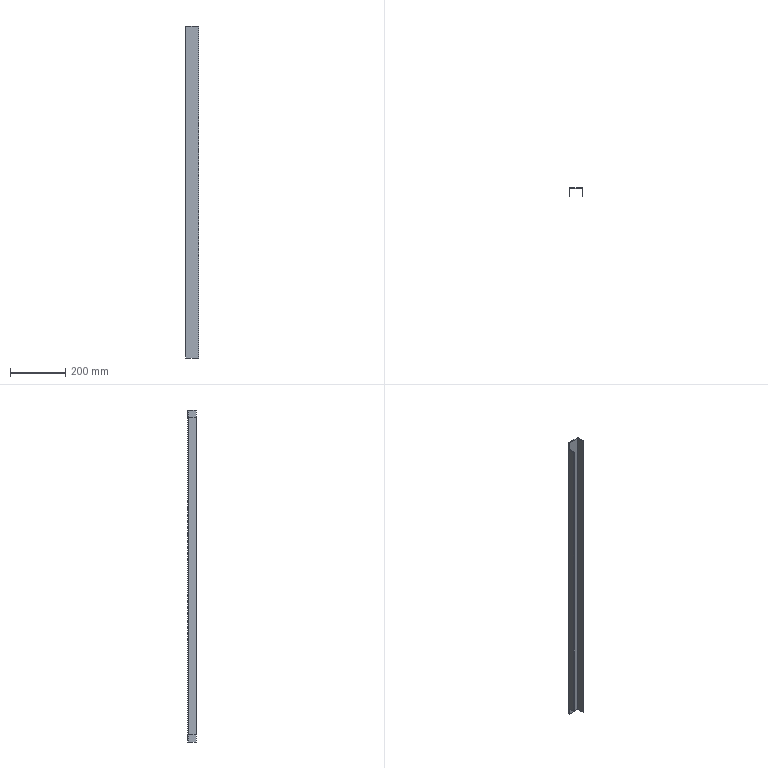Part | SolidWorks | 1 solid | 26 faces | box 50 x 30 x 1204 mm | volume 365931 mm3 | plane 22 | cylinder 4 | commonest cylinder face diameters 0.2 x2 6.2 x2
STEP:
#1=CARTESIAN_POINT('',(-25.,-3.1,575.));
#2=VERTEX_POINT('',#1);
#3=CARTESIAN_POINT('',(-25.,-30.,575.));
#4=VERTEX_POINT('',#3);
#5=CARTESIAN_POINT('',(-25.,-30.,575.));
#6=DIRECTION('',(0.,-1.,0.));
#7=VECTOR('',#6,1000.);
#8=LINE('',#5,#7);
#9=EDGE_CURVE('',#2,#4,#8,.T.);
#10=ORIENTED_EDGE('',*,*,#9,.F.);
#11=CARTESIAN_POINT('',(-25.,-3.1,-575.));
#12=VERTEX_POINT('',#11);
#13=CARTESIAN_POINT('',(-25.,-3.1,-602.));
#14=DIRECTION('',(0.,0.,1.));
#15=VECTOR('',#14,1000.);
#16=LINE('',#13,#15);
#17=EDGE_CURVE('',#12,#2,#16,.T.);
#18=ORIENTED_EDGE('',*,*,#17,.F.);
#19=CARTESIAN_POINT('',(-25.,-30.,-575.));
#20=VERTEX_POINT('',#19);
#21=CARTESIAN_POINT('',(-25.,-30.,-575.));
#22=DIRECTION('',(0.,-1.,0.));
#23=VECTOR('',#22,1000.);
#24=LINE('',#21,#23);
#25=EDGE_CURVE('',#12,#20,#24,.T.);
#26=ORIENTED_EDGE('',*,*,#25,.T.);
#27=CARTESIAN_POINT('',(-25.,-30.,-602.));
#28=DIRECTION('',(0.,0.,1.));
#29=VECTOR('',#28,1000.);
#30=LINE('',#27,#29);
#31=EDGE_CURVE('',#20,#4,#30,.T.);
#32=ORIENTED_EDGE('',*,*,#31,.T.);
#33=EDGE_LOOP('',(#10,#18,#26,#32));
#34=FACE_OUTER_BOUND('',#33,.T.);
#35=CARTESIAN_POINT('',(-25.,0.,-602.));
#36=DIRECTION('',(1.,0.,0.));
#37=DIRECTION('',(0.,0.,1.));
#38=AXIS2_PLACEMENT_3D('',#35,#36,#37);
#39=PLANE('',#38);
#40=ADVANCED_FACE('',(#34),#39,.F.);
#41=ORIENTED_EDGE('',*,*,#31,.F.);
#42=CARTESIAN_POINT('',(-22.,-30.,-575.));
#43=VERTEX_POINT('',#42);
#44=CARTESIAN_POINT('',(-25.,-30.,-575.));
#45=DIRECTION('',(1.,0.,0.));
#46=VECTOR('',#45,1000.);
#47=LINE('',#44,#46);
#48=EDGE_CURVE('',#20,#43,#47,.T.);
#49=ORIENTED_EDGE('',*,*,#48,.T.);
#50=CARTESIAN_POINT('',(-22.,-30.,575.));
#51=VERTEX_POINT('',#50);
#52=CARTESIAN_POINT('',(-22.,-30.,-602.));
#53=DIRECTION('',(0.,0.,1.));
#54=VECTOR('',#53,1000.);
#55=LINE('',#52,#54);
#56=EDGE_CURVE('',#43,#51,#55,.T.);
#57=ORIENTED_EDGE('',*,*,#56,.T.);
#58=CARTESIAN_POINT('',(-25.,-30.,575.));
#59=DIRECTION('',(1.,0.,0.));
#60=VECTOR('',#59,1000.);
#61=LINE('',#58,#60);
#62=EDGE_CURVE('',#4,#51,#61,.T.);
#63=ORIENTED_EDGE('',*,*,#62,.F.);
#64=EDGE_LOOP('',(#41,#49,#57,#63));
#65=FACE_OUTER_BOUND('',#64,.T.);
#66=CARTESIAN_POINT('',(-22.,-30.,-602.));
#67=DIRECTION('',(0.,-1.,0.));
#68=DIRECTION('',(0.,0.,1.));
#69=AXIS2_PLACEMENT_3D('',#66,#67,#68);
#70=PLANE('',#69);
#71=ADVANCED_FACE('',(#65),#70,.T.);
#72=ORIENTED_EDGE('',*,*,#56,.F.);
#73=CARTESIAN_POINT('',(-22.,-3.1,-575.));
#74=VERTEX_POINT('',#73);
#75=CARTESIAN_POINT('',(-22.,0.,-575.));
#76=DIRECTION('',(0.,-1.,0.));
#77=VECTOR('',#76,1000.);
#78=LINE('',#75,#77);
#79=EDGE_CURVE('',#74,#43,#78,.T.);
#80=ORIENTED_EDGE('',*,*,#79,.F.);
#81=CARTESIAN_POINT('',(-22.,-3.1,575.));
#82=VERTEX_POINT('',#81);
#83=CARTESIAN_POINT('',(-22.,-3.1,-602.));
#84=DIRECTION('',(0.,0.,1.));
#85=VECTOR('',#84,1000.);
#86=LINE('',#83,#85);
#87=EDGE_CURVE('',#74,#82,#86,.T.);
#88=ORIENTED_EDGE('',*,*,#87,.T.);
#89=CARTESIAN_POINT('',(-22.,0.,575.));
#90=DIRECTION('',(0.,-1.,0.));
#91=VECTOR('',#90,1000.);
#92=LINE('',#89,#91);
#93=EDGE_CURVE('',#82,#51,#92,.T.);
#94=ORIENTED_EDGE('',*,*,#93,.T.);
#95=EDGE_LOOP('',(#72,#80,#88,#94));
#96=FACE_OUTER_BOUND('',#95,.T.);
#97=CARTESIAN_POINT('',(-22.,0.,-602.));
#98=DIRECTION('',(1.,0.,0.));
#99=DIRECTION('',(0.,0.,1.));
#100=AXIS2_PLACEMENT_3D('',#97,#98,#99);
#101=PLANE('',#100);
#102=ADVANCED_FACE('',(#96),#101,.T.);
#103=CARTESIAN_POINT('',(-21.903,-3.,575.));
#104=VERTEX_POINT('',#103);
#105=CARTESIAN_POINT('',(-21.9,-3.1,575.));
#106=DIRECTION('',(0.,0.,-1.));
#107=DIRECTION('',(-1.,0.,0.));
#108=AXIS2_PLACEMENT_3D('',#105,#106,#107);
#109=CIRCLE('',#108,0.1);
#110=EDGE_CURVE('',#82,#104,#109,.T.);
#111=ORIENTED_EDGE('',*,*,#110,.F.);
#112=ORIENTED_EDGE('',*,*,#87,.F.);
#113=CARTESIAN_POINT('',(-21.903,-3.,-575.));
#114=VERTEX_POINT('',#113);
#115=CARTESIAN_POINT('',(-21.9,-3.1,-575.));
#116=DIRECTION('',(0.,0.,-1.));
#117=DIRECTION('',(-1.,0.,0.));
#118=AXIS2_PLACEMENT_3D('',#115,#116,#117);
#119=CIRCLE('',#118,0.1);
#120=EDGE_CURVE('',#74,#114,#119,.T.);
#121=ORIENTED_EDGE('',*,*,#120,.T.);
#122=CARTESIAN_POINT('',(-21.903,-3.,-602.));
#123=VERTEX_POINT('',#122);
#124=CARTESIAN_POINT('',(-21.903,-3.,-602.));
#125=DIRECTION('',(0.,0.,1.));
#126=VECTOR('',#125,1000.);
#127=LINE('',#124,#126);
#128=EDGE_CURVE('',#123,#114,#127,.T.);
#129=ORIENTED_EDGE('',*,*,#128,.F.);
#130=CARTESIAN_POINT('',(-21.9,-3.,-602.));
#131=VERTEX_POINT('',#130);
#132=CARTESIAN_POINT('',(-21.9,-3.1,-602.));
#133=DIRECTION('',(0.,0.,1.));
#134=DIRECTION('',(1.,0.,0.));
#135=AXIS2_PLACEMENT_3D('',#132,#133,#134);
#136=CIRCLE('',#135,0.1);
#137=EDGE_CURVE('',#131,#123,#136,.T.);
#138=ORIENTED_EDGE('',*,*,#137,.F.);
#139=CARTESIAN_POINT('',(-21.9,-3.,602.));
#140=VERTEX_POINT('',#139);
#141=CARTESIAN_POINT('',(-21.9,-3.,-602.));
#142=DIRECTION('',(0.,0.,1.));
#143=VECTOR('',#142,1000.);
#144=LINE('',#141,#143);
#145=EDGE_CURVE('',#131,#140,#144,.T.);
#146=ORIENTED_EDGE('',*,*,#145,.T.);
#147=CARTESIAN_POINT('',(-21.903,-3.,602.));
#148=VERTEX_POINT('',#147);
#149=CARTESIAN_POINT('',(-21.9,-3.1,602.));
#150=DIRECTION('',(0.,0.,1.));
#151=DIRECTION('',(1.,0.,0.));
#152=AXIS2_PLACEMENT_3D('',#149,#150,#151);
#153=CIRCLE('',#152,0.1);
#154=EDGE_CURVE('',#140,#148,#153,.T.);
#155=ORIENTED_EDGE('',*,*,#154,.T.);
#156=CARTESIAN_POINT('',(-21.903,-3.,-602.));
#157=DIRECTION('',(0.,0.,1.));
#158=VECTOR('',#157,1000.);
#159=LINE('',#156,#158);
#160=EDGE_CURVE('',#104,#148,#159,.T.);
#161=ORIENTED_EDGE('',*,*,#160,.F.);
#162=EDGE_LOOP('',(#111,#112,#121,#129,#138,#146,#155,#161));
#163=FACE_OUTER_BOUND('',#162,.T.);
#164=CARTESIAN_POINT('',(-21.9,-3.1,-602.));
#165=DIRECTION('',(0.,0.,1.));
#166=DIRECTION('',(-1.,0.,0.));
#167=AXIS2_PLACEMENT_3D('',#164,#165,#166);
#168=CYLINDRICAL_SURFACE('',#167,0.1);
#169=ADVANCED_FACE('',(#163),#168,.F.);
#170=CARTESIAN_POINT('',(-22.,-0.001613,575.));
#171=VERTEX_POINT('',#170);
#172=CARTESIAN_POINT('',(-22.,-0.001613,602.));
#173=VERTEX_POINT('',#172);
#174=CARTESIAN_POINT('',(-22.,-0.001613,-602.));
#175=DIRECTION('',(0.,0.,1.));
#176=VECTOR('',#175,1000.);
#177=LINE('',#174,#176);
#178=EDGE_CURVE('',#171,#173,#177,.T.);
#179=ORIENTED_EDGE('',*,*,#178,.T.);
#180=CARTESIAN_POINT('',(-21.9,0.,602.));
#181=VERTEX_POINT('',#180);
#182=CARTESIAN_POINT('',(-21.9,-3.1,602.));
#183=DIRECTION('',(0.,0.,1.));
#184=DIRECTION('',(-1.,0.,0.));
#185=AXIS2_PLACEMENT_3D('',#182,#183,#184);
#186=CIRCLE('',#185,3.1);
#187=EDGE_CURVE('',#181,#173,#186,.T.);
#188=ORIENTED_EDGE('',*,*,#187,.F.);
#189=CARTESIAN_POINT('',(-21.9,0.,-602.));
#190=VERTEX_POINT('',#189);
#191=CARTESIAN_POINT('',(-21.9,0.,-602.));
#192=DIRECTION('',(0.,0.,1.));
#193=VECTOR('',#192,1000.);
#194=LINE('',#191,#193);
#195=EDGE_CURVE('',#190,#181,#194,.T.);
#196=ORIENTED_EDGE('',*,*,#195,.F.);
#197=CARTESIAN_POINT('',(-22.,-0.001613,-602.));
#198=VERTEX_POINT('',#197);
#199=CARTESIAN_POINT('',(-21.9,-3.1,-602.));
#200=DIRECTION('',(0.,0.,1.));
#201=DIRECTION('',(-1.,0.,0.));
#202=AXIS2_PLACEMENT_3D('',#199,#200,#201);
#203=CIRCLE('',#202,3.1);
#204=EDGE_CURVE('',#190,#198,#203,.T.);
#205=ORIENTED_EDGE('',*,*,#204,.T.);
#206=CARTESIAN_POINT('',(-22.,-0.001613,-575.));
#207=VERTEX_POINT('',#206);
#208=CARTESIAN_POINT('',(-22.,-0.001613,-602.));
#209=DIRECTION('',(0.,0.,1.));
#210=VECTOR('',#209,1000.);
#211=LINE('',#208,#210);
#212=EDGE_CURVE('',#198,#207,#211,.T.);
#213=ORIENTED_EDGE('',*,*,#212,.T.);
#214=CARTESIAN_POINT('',(-21.9,-3.1,-575.));
#215=DIRECTION('',(0.,0.,-1.));
#216=DIRECTION('',(-1.,0.,0.));
#217=AXIS2_PLACEMENT_3D('',#214,#215,#216);
#218=CIRCLE('',#217,3.1);
#219=EDGE_CURVE('',#12,#207,#218,.T.);
#220=ORIENTED_EDGE('',*,*,#219,.F.);
#221=ORIENTED_EDGE('',*,*,#17,.T.);
#222=CARTESIAN_POINT('',(-21.9,-3.1,575.));
#223=DIRECTION('',(0.,0.,-1.));
#224=DIRECTION('',(-1.,0.,0.));
#225=AXIS2_PLACEMENT_3D('',#222,#223,#224);
#226=CIRCLE('',#225,3.1);
#227=EDGE_CURVE('',#2,#171,#226,.T.);
#228=ORIENTED_EDGE('',*,*,#227,.T.);
#229=EDGE_LOOP('',(#179,#188,#196,#205,#213,#220,#221,#228));
#230=FACE_OUTER_BOUND('',#229,.T.);
#231=CARTESIAN_POINT('',(-21.9,-3.1,-602.));
#232=DIRECTION('',(0.,0.,1.));
#233=DIRECTION('',(-1.,0.,0.));
#234=AXIS2_PLACEMENT_3D('',#231,#232,#233);
#235=CYLINDRICAL_SURFACE('',#234,3.1);
#236=ADVANCED_FACE('',(#230),#235,.T.);
#237=ORIENTED_EDGE('',*,*,#154,.F.);
#238=CARTESIAN_POINT('',(-21.9,-3.,602.));
#239=DIRECTION('',(0.,1.,0.));
#240=VECTOR('',#239,1000.);
#241=LINE('',#238,#240);
#242=EDGE_CURVE('',#140,#181,#241,.T.);
#243=ORIENTED_EDGE('',*,*,#242,.T.);
#244=ORIENTED_EDGE('',*,*,#187,.T.);
#245=CARTESIAN_POINT('',(-22.,-0.001613,602.));
#246=DIRECTION('',(0.03226,-0.9995,0.));
#247=VECTOR('',#246,1000.);
#248=LINE('',#245,#247);
#249=EDGE_CURVE('',#173,#148,#248,.T.);
#250=ORIENTED_EDGE('',*,*,#249,.T.);
#251=EDGE_LOOP('',(#237,#243,#244,#250));
#252=FACE_OUTER_BOUND('',#251,.T.);
#253=CARTESIAN_POINT('',(-25.,-3.1,602.));
#254=DIRECTION('',(0.,0.,1.));
#255=DIRECTION('',(-1.,0.,0.));
#256=AXIS2_PLACEMENT_3D('',#253,#254,#255);
#257=PLANE('',#256);
#258=ADVANCED_FACE('',(#252),#257,.T.);
#259=ORIENTED_EDGE('',*,*,#204,.F.);
#260=CARTESIAN_POINT('',(-21.9,0.,-602.));
#261=DIRECTION('',(0.,-1.,0.));
#262=VECTOR('',#261,1000.);
#263=LINE('',#260,#262);
#264=EDGE_CURVE('',#190,#131,#263,.T.);
#265=ORIENTED_EDGE('',*,*,#264,.T.);
#266=ORIENTED_EDGE('',*,*,#137,.T.);
#267=CARTESIAN_POINT('',(-22.,-0.001613,-602.));
#268=DIRECTION('',(0.03226,-0.9995,0.));
#269=VECTOR('',#268,1000.);
#270=LINE('',#267,#269);
#271=EDGE_CURVE('',#198,#123,#270,.T.);
#272=ORIENTED_EDGE('',*,*,#271,.F.);
#273=EDGE_LOOP('',(#259,#265,#266,#272));
#274=FACE_OUTER_BOUND('',#273,.T.);
#275=CARTESIAN_POINT('',(-21.9,0.,-602.));
#276=DIRECTION('',(0.,0.,-1.));
#277=DIRECTION('',(1.,0.,0.));
#278=AXIS2_PLACEMENT_3D('',#275,#276,#277);
#279=PLANE('',#278);
#280=ADVANCED_FACE('',(#274),#279,.T.);
#281=CARTESIAN_POINT('',(25.,-3.1,-602.));
#282=VERTEX_POINT('',#281);
#283=CARTESIAN_POINT('',(22.,-3.1,-602.));
#284=VERTEX_POINT('',#283);
#285=CARTESIAN_POINT('',(25.,-3.1,-602.));
#286=DIRECTION('',(-1.,0.,0.));
#287=VECTOR('',#286,1000.);
#288=LINE('',#285,#287);
#289=EDGE_CURVE('',#282,#284,#288,.T.);
#290=ORIENTED_EDGE('',*,*,#289,.T.);
#291=CARTESIAN_POINT('',(21.9,-3.,-602.));
#292=VERTEX_POINT('',#291);
#293=CARTESIAN_POINT('',(21.9,-3.1,-602.));
#294=DIRECTION('',(0.,0.,1.));
#295=DIRECTION('',(1.,0.,0.));
#296=AXIS2_PLACEMENT_3D('',#293,#294,#295);
#297=CIRCLE('',#296,0.1);
#298=EDGE_CURVE('',#284,#292,#297,.T.);
#299=ORIENTED_EDGE('',*,*,#298,.T.);
#300=CARTESIAN_POINT('',(21.9,0.,-602.));
#301=VERTEX_POINT('',#300);
#302=CARTESIAN_POINT('',(21.9,-3.,-602.));
#303=DIRECTION('',(0.,1.,0.));
#304=VECTOR('',#303,1000.);
#305=LINE('',#302,#304);
#306=EDGE_CURVE('',#292,#301,#305,.T.);
#307=ORIENTED_EDGE('',*,*,#306,.T.);
#308=CARTESIAN_POINT('',(21.9,-3.1,-602.));
#309=DIRECTION('',(0.,0.,1.));
#310=DIRECTION('',(-1.,0.,0.));
#311=AXIS2_PLACEMENT_3D('',#308,#309,#310);
#312=CIRCLE('',#311,3.1);
#313=EDGE_CURVE('',#282,#301,#312,.T.);
#314=ORIENTED_EDGE('',*,*,#313,.F.);
#315=EDGE_LOOP('',(#290,#299,#307,#314));
#316=FACE_OUTER_BOUND('',#315,.T.);
#317=CARTESIAN_POINT('',(25.,-3.1,-602.));
#318=DIRECTION('',(0.,0.,-1.));
#319=DIRECTION('',(1.,0.,0.));
#320=AXIS2_PLACEMENT_3D('',#317,#318,#319);
#321=PLANE('',#320);
#322=ADVANCED_FACE('',(#316),#321,.T.);
#323=CARTESIAN_POINT('',(25.,-30.,-602.));
#324=VERTEX_POINT('',#323);
#325=CARTESIAN_POINT('',(25.,0.,-602.));
#326=DIRECTION('',(0.,1.,0.));
#327=VECTOR('',#326,1000.);
#328=LINE('',#325,#327);
#329=EDGE_CURVE('',#324,#282,#328,.T.);
#330=ORIENTED_EDGE('',*,*,#329,.F.);
#331=CARTESIAN_POINT('',(22.,-30.,-602.));
#332=VERTEX_POINT('',#331);
#333=CARTESIAN_POINT('',(25.,-30.,-602.));
#334=DIRECTION('',(-1.,0.,0.));
#335=VECTOR('',#334,1000.);
#336=LINE('',#333,#335);
#337=EDGE_CURVE('',#324,#332,#336,.T.);
#338=ORIENTED_EDGE('',*,*,#337,.T.);
#339=CARTESIAN_POINT('',(22.,0.,-602.));
#340=DIRECTION('',(0.,1.,0.));
#341=VECTOR('',#340,1000.);
#342=LINE('',#339,#341);
#343=EDGE_CURVE('',#332,#284,#342,.T.);
#344=ORIENTED_EDGE('',*,*,#343,.T.);
#345=ORIENTED_EDGE('',*,*,#289,.F.);
#346=EDGE_LOOP('',(#330,#338,#344,#345));
#347=FACE_OUTER_BOUND('',#346,.T.);
#348=CARTESIAN_POINT('',(21.9,-3.,-602.));
#349=DIRECTION('',(0.,0.,-1.));
#350=DIRECTION('',(1.,0.,0.));
#351=AXIS2_PLACEMENT_3D('',#348,#349,#350);
#352=PLANE('',#351);
#353=ADVANCED_FACE('',(#347),#352,.T.);
#354=CARTESIAN_POINT('',(21.9,0.,602.));
#355=VERTEX_POINT('',#354);
#356=CARTESIAN_POINT('',(21.9,-3.,602.));
#357=VERTEX_POINT('',#356);
#358=CARTESIAN_POINT('',(21.9,0.,602.));
#359=DIRECTION('',(0.,-1.,0.));
#360=VECTOR('',#359,1000.);
#361=LINE('',#358,#360);
#362=EDGE_CURVE('',#355,#357,#361,.T.);
#363=ORIENTED_EDGE('',*,*,#362,.T.);
#364=CARTESIAN_POINT('',(22.,-3.1,602.));
#365=VERTEX_POINT('',#364);
#366=CARTESIAN_POINT('',(21.9,-3.1,602.));
#367=DIRECTION('',(0.,0.,1.));
#368=DIRECTION('',(1.,0.,0.));
#369=AXIS2_PLACEMENT_3D('',#366,#367,#368);
#370=CIRCLE('',#369,0.1);
#371=EDGE_CURVE('',#365,#357,#370,.T.);
#372=ORIENTED_EDGE('',*,*,#371,.F.);
#373=CARTESIAN_POINT('',(25.,-3.1,602.));
#374=VERTEX_POINT('',#373);
#375=CARTESIAN_POINT('',(22.,-3.1,602.));
#376=DIRECTION('',(1.,0.,0.));
#377=VECTOR('',#376,1000.);
#378=LINE('',#375,#377);
#379=EDGE_CURVE('',#365,#374,#378,.T.);
#380=ORIENTED_EDGE('',*,*,#379,.T.);
#381=CARTESIAN_POINT('',(21.9,-3.1,602.));
#382=DIRECTION('',(0.,0.,1.));
#383=DIRECTION('',(-1.,0.,0.));
#384=AXIS2_PLACEMENT_3D('',#381,#382,#383);
#385=CIRCLE('',#384,3.1);
#386=EDGE_CURVE('',#374,#355,#385,.T.);
#387=ORIENTED_EDGE('',*,*,#386,.T.);
#388=EDGE_LOOP('',(#363,#372,#380,#387));
#389=FACE_OUTER_BOUND('',#388,.T.);
#390=CARTESIAN_POINT('',(21.9,0.,602.));
#391=DIRECTION('',(0.,0.,1.));
#392=DIRECTION('',(-1.,0.,0.));
#393=AXIS2_PLACEMENT_3D('',#390,#391,#392);
#394=PLANE('',#393);
#395=ADVANCED_FACE('',(#389),#394,.T.);
#396=CARTESIAN_POINT('',(-25.,0.,602.));
#397=DIRECTION('',(-1.,0.,0.));
#398=VECTOR('',#397,1000.);
#399=LINE('',#396,#398);
#400=EDGE_CURVE('',#355,#181,#399,.T.);
#401=ORIENTED_EDGE('',*,*,#400,.T.);
#402=ORIENTED_EDGE('',*,*,#242,.F.);
#403=CARTESIAN_POINT('',(-25.,-3.,602.));
#404=DIRECTION('',(-1.,0.,0.));
#405=VECTOR('',#404,1000.);
#406=LINE('',#403,#405);
#407=EDGE_CURVE('',#357,#140,#406,.T.);
#408=ORIENTED_EDGE('',*,*,#407,.F.);
#409=ORIENTED_EDGE('',*,*,#362,.F.);
#410=EDGE_LOOP('',(#401,#402,#408,#409));
#411=FACE_OUTER_BOUND('',#410,.T.);
#412=CARTESIAN_POINT('',(22.,-3.1,602.));
#413=DIRECTION('',(0.,0.,1.));
#414=DIRECTION('',(-1.,0.,0.));
#415=AXIS2_PLACEMENT_3D('',#412,#413,#414);
#416=PLANE('',#415);
#417=ADVANCED_FACE('',(#411),#416,.T.);
#418=CARTESIAN_POINT('',(-25.,0.,-602.));
#419=DIRECTION('',(-1.,0.,0.));
#420=VECTOR('',#419,1000.);
#421=LINE('',#418,#420);
#422=EDGE_CURVE('',#301,#190,#421,.T.);
#423=ORIENTED_EDGE('',*,*,#422,.F.);
#424=ORIENTED_EDGE('',*,*,#306,.F.);
#425=CARTESIAN_POINT('',(-25.,-3.,-602.));
#426=DIRECTION('',(-1.,0.,0.));
#427=VECTOR('',#426,1000.);
#428=LINE('',#425,#427);
#429=EDGE_CURVE('',#292,#131,#428,.T.);
#430=ORIENTED_EDGE('',*,*,#429,.T.);
#431=ORIENTED_EDGE('',*,*,#264,.F.);
#432=EDGE_LOOP('',(#423,#424,#430,#431));
#433=FACE_OUTER_BOUND('',#432,.T.);
#434=CARTESIAN_POINT('',(-22.,-3.1,-602.));
#435=DIRECTION('',(0.,0.,-1.));
#436=DIRECTION('',(1.,0.,0.));
#437=AXIS2_PLACEMENT_3D('',#434,#435,#436);
#438=PLANE('',#437);
#439=ADVANCED_FACE('',(#433),#438,.T.);
#440=ORIENTED_EDGE('',*,*,#407,.T.);
#441=ORIENTED_EDGE('',*,*,#145,.F.);
#442=ORIENTED_EDGE('',*,*,#429,.F.);
#443=CARTESIAN_POINT('',(21.9,-3.,-602.));
#444=DIRECTION('',(0.,0.,1.));
#445=VECTOR('',#444,1000.);
#446=LINE('',#443,#445);
#447=EDGE_CURVE('',#292,#357,#446,.T.);
#448=ORIENTED_EDGE('',*,*,#447,.T.);
#449=EDGE_LOOP('',(#440,#441,#442,#448));
#450=FACE_OUTER_BOUND('',#449,.T.);
#451=CARTESIAN_POINT('',(-25.,-3.,-602.));
#452=DIRECTION('',(0.,-1.,0.));
#453=DIRECTION('',(1.,0.,0.));
#454=AXIS2_PLACEMENT_3D('',#451,#452,#453);
#455=PLANE('',#454);
#456=ADVANCED_FACE('',(#450),#455,.T.);
#457=ORIENTED_EDGE('',*,*,#371,.T.);
#458=ORIENTED_EDGE('',*,*,#447,.F.);
#459=ORIENTED_EDGE('',*,*,#298,.F.);
#460=CARTESIAN_POINT('',(22.,-3.1,-602.));
#461=DIRECTION('',(0.,0.,1.));
#462=VECTOR('',#461,1000.);
#463=LINE('',#460,#462);
#464=EDGE_CURVE('',#284,#365,#463,.T.);
#465=ORIENTED_EDGE('',*,*,#464,.T.);
#466=EDGE_LOOP('',(#457,#458,#459,#465));
#467=FACE_OUTER_BOUND('',#466,.T.);
#468=CARTESIAN_POINT('',(21.9,-3.1,-602.));
#469=DIRECTION('',(0.,0.,1.));
#470=DIRECTION('',(-1.,0.,0.));
#471=AXIS2_PLACEMENT_3D('',#468,#469,#470);
#472=CYLINDRICAL_SURFACE('',#471,0.1);
#473=ADVANCED_FACE('',(#467),#472,.F.);
#474=CARTESIAN_POINT('',(22.,-30.,602.));
#475=VERTEX_POINT('',#474);
#476=CARTESIAN_POINT('',(22.,0.,602.));
#477=DIRECTION('',(0.,1.,0.));
#478=VECTOR('',#477,1000.);
#479=LINE('',#476,#478);
#480=EDGE_CURVE('',#475,#365,#479,.T.);
#481=ORIENTED_EDGE('',*,*,#480,.T.);
#482=ORIENTED_EDGE('',*,*,#464,.F.);
#483=ORIENTED_EDGE('',*,*,#343,.F.);
#484=CARTESIAN_POINT('',(22.,-30.,-602.));
#485=DIRECTION('',(0.,0.,1.));
#486=VECTOR('',#485,1000.);
#487=LINE('',#484,#486);
#488=EDGE_CURVE('',#332,#475,#487,.T.);
#489=ORIENTED_EDGE('',*,*,#488,.T.);
#490=EDGE_LOOP('',(#481,#482,#483,#489));
#491=FACE_OUTER_BOUND('',#490,.T.);
#492=CARTESIAN_POINT('',(22.,0.,-602.));
#493=DIRECTION('',(-1.,0.,0.));
#494=DIRECTION('',(0.,-1.,0.));
#495=AXIS2_PLACEMENT_3D('',#492,#493,#494);
#496=PLANE('',#495);
#497=ADVANCED_FACE('',(#491),#496,.T.);
#498=CARTESIAN_POINT('',(25.,-30.,602.));
#499=VERTEX_POINT('',#498);
#500=CARTESIAN_POINT('',(25.,-30.,602.));
#501=DIRECTION('',(-1.,0.,0.));
#502=VECTOR('',#501,1000.);
#503=LINE('',#500,#502);
#504=EDGE_CURVE('',#499,#475,#503,.T.);
#505=ORIENTED_EDGE('',*,*,#504,.T.);
#506=ORIENTED_EDGE('',*,*,#488,.F.);
#507=ORIENTED_EDGE('',*,*,#337,.F.);
#508=CARTESIAN_POINT('',(25.,-30.,-602.));
#509=DIRECTION('',(0.,0.,1.));
#510=VECTOR('',#509,1000.);
#511=LINE('',#508,#510);
#512=EDGE_CURVE('',#324,#499,#511,.T.);
#513=ORIENTED_EDGE('',*,*,#512,.T.);
#514=EDGE_LOOP('',(#505,#506,#507,#513));
#515=FACE_OUTER_BOUND('',#514,.T.);
#516=CARTESIAN_POINT('',(25.,-30.,-602.));
#517=DIRECTION('',(0.,-1.,0.));
#518=DIRECTION('',(1.,0.,0.));
#519=AXIS2_PLACEMENT_3D('',#516,#517,#518);
#520=PLANE('',#519);
#521=ADVANCED_FACE('',(#515),#520,.T.);
#522=CARTESIAN_POINT('',(25.,0.,602.));
#523=DIRECTION('',(0.,1.,0.));
#524=VECTOR('',#523,1000.);
#525=LINE('',#522,#524);
#526=EDGE_CURVE('',#499,#374,#525,.T.);
#527=ORIENTED_EDGE('',*,*,#526,.F.);
#528=ORIENTED_EDGE('',*,*,#512,.F.);
#529=ORIENTED_EDGE('',*,*,#329,.T.);
#530=CARTESIAN_POINT('',(25.,-3.1,-602.));
#531=DIRECTION('',(0.,0.,1.));
#532=VECTOR('',#531,1000.);
#533=LINE('',#530,#532);
#534=EDGE_CURVE('',#282,#374,#533,.T.);
#535=ORIENTED_EDGE('',*,*,#534,.T.);
#536=EDGE_LOOP('',(#527,#528,#529,#535));
#537=FACE_OUTER_BOUND('',#536,.T.);
#538=CARTESIAN_POINT('',(25.,0.,-602.));
#539=DIRECTION('',(-1.,0.,0.));
#540=DIRECTION('',(0.,-1.,0.));
#541=AXIS2_PLACEMENT_3D('',#538,#539,#540);
#542=PLANE('',#541);
#543=ADVANCED_FACE('',(#537),#542,.F.);
#544=ORIENTED_EDGE('',*,*,#386,.F.);
#545=ORIENTED_EDGE('',*,*,#534,.F.);
#546=ORIENTED_EDGE('',*,*,#313,.T.);
#547=CARTESIAN_POINT('',(21.9,0.,-602.));
#548=DIRECTION('',(0.,0.,1.));
#549=VECTOR('',#548,1000.);
#550=LINE('',#547,#549);
#551=EDGE_CURVE('',#301,#355,#550,.T.);
#552=ORIENTED_EDGE('',*,*,#551,.T.);
#553=EDGE_LOOP('',(#544,#545,#546,#552));
#554=FACE_OUTER_BOUND('',#553,.T.);
#555=CARTESIAN_POINT('',(21.9,-3.1,-602.));
#556=DIRECTION('',(0.,0.,1.));
#557=DIRECTION('',(-1.,0.,0.));
#558=AXIS2_PLACEMENT_3D('',#555,#556,#557);
#559=CYLINDRICAL_SURFACE('',#558,3.1);
#560=ADVANCED_FACE('',(#554),#559,.T.);
#561=ORIENTED_EDGE('',*,*,#400,.F.);
#562=ORIENTED_EDGE('',*,*,#551,.F.);
#563=ORIENTED_EDGE('',*,*,#422,.T.);
#564=ORIENTED_EDGE('',*,*,#195,.T.);
#565=EDGE_LOOP('',(#561,#562,#563,#564));
#566=FACE_OUTER_BOUND('',#565,.T.);
#567=CARTESIAN_POINT('',(-25.,0.,-602.));
#568=DIRECTION('',(0.,-1.,0.));
#569=DIRECTION('',(1.,0.,0.));
#570=AXIS2_PLACEMENT_3D('',#567,#568,#569);
#571=PLANE('',#570);
#572=ADVANCED_FACE('',(#566),#571,.F.);
#573=ORIENTED_EDGE('',*,*,#480,.F.);
#574=ORIENTED_EDGE('',*,*,#504,.F.);
#575=ORIENTED_EDGE('',*,*,#526,.T.);
#576=ORIENTED_EDGE('',*,*,#379,.F.);
#577=EDGE_LOOP('',(#573,#574,#575,#576));
#578=FACE_OUTER_BOUND('',#577,.T.);
#579=CARTESIAN_POINT('',(-21.9,-3.1,602.));
#580=DIRECTION('',(0.,0.,-1.));
#581=DIRECTION('',(1.,0.,0.));
#582=AXIS2_PLACEMENT_3D('',#579,#580,#581);
#583=PLANE('',#582);
#584=ADVANCED_FACE('',(#578),#583,.F.);
#585=CARTESIAN_POINT('',(-25.,-3.1,-575.));
#586=DIRECTION('',(1.,0.,0.));
#587=VECTOR('',#586,1000.);
#588=LINE('',#585,#587);
#589=EDGE_CURVE('',#12,#74,#588,.T.);
#590=ORIENTED_EDGE('',*,*,#589,.T.);
#591=ORIENTED_EDGE('',*,*,#79,.T.);
#592=ORIENTED_EDGE('',*,*,#48,.F.);
#593=ORIENTED_EDGE('',*,*,#25,.F.);
#594=EDGE_LOOP('',(#590,#591,#592,#593));
#595=FACE_OUTER_BOUND('',#594,.T.);
#596=CARTESIAN_POINT('',(-25.,-30.,-575.));
#597=DIRECTION('',(0.,0.,-1.));
#598=DIRECTION('',(0.,-1.,0.));
#599=AXIS2_PLACEMENT_3D('',#596,#597,#598);
#600=PLANE('',#599);
#601=ADVANCED_FACE('',(#595),#600,.T.);
#602=ORIENTED_EDGE('',*,*,#271,.T.);
#603=ORIENTED_EDGE('',*,*,#128,.T.);
#604=CARTESIAN_POINT('',(-22.,-0.001613,-575.));
#605=DIRECTION('',(0.03226,-0.9995,0.));
#606=VECTOR('',#605,1000.);
#607=LINE('',#604,#606);
#608=EDGE_CURVE('',#207,#114,#607,.T.);
#609=ORIENTED_EDGE('',*,*,#608,.F.);
#610=ORIENTED_EDGE('',*,*,#212,.F.);
#611=EDGE_LOOP('',(#602,#603,#609,#610));
#612=FACE_OUTER_BOUND('',#611,.T.);
#613=CARTESIAN_POINT('',(-22.,-0.001613,-588.5));
#614=DIRECTION('',(0.9995,0.03226,0.));
#615=DIRECTION('',(0.,0.,1.));
#616=AXIS2_PLACEMENT_3D('',#613,#614,#615);
#617=PLANE('',#616);
#618=ADVANCED_FACE('',(#612),#617,.F.);
#619=ORIENTED_EDGE('',*,*,#608,.T.);
#620=ORIENTED_EDGE('',*,*,#120,.F.);
#621=ORIENTED_EDGE('',*,*,#589,.F.);
#622=ORIENTED_EDGE('',*,*,#219,.T.);
#623=EDGE_LOOP('',(#619,#620,#621,#622));
#624=FACE_OUTER_BOUND('',#623,.T.);
#625=CARTESIAN_POINT('',(-21.9,-3.1,-575.));
#626=DIRECTION('',(0.,0.,-1.));
#627=DIRECTION('',(1.,0.,0.));
#628=AXIS2_PLACEMENT_3D('',#625,#626,#627);
#629=PLANE('',#628);
#630=ADVANCED_FACE('',(#624),#629,.T.);
#631=ORIENTED_EDGE('',*,*,#9,.T.);
#632=ORIENTED_EDGE('',*,*,#62,.T.);
#633=ORIENTED_EDGE('',*,*,#93,.F.);
#634=CARTESIAN_POINT('',(-25.,-3.1,575.));
#635=DIRECTION('',(1.,0.,0.));
#636=VECTOR('',#635,1000.);
#637=LINE('',#634,#636);
#638=EDGE_CURVE('',#2,#82,#637,.T.);
#639=ORIENTED_EDGE('',*,*,#638,.F.);
#640=EDGE_LOOP('',(#631,#632,#633,#639));
#641=FACE_OUTER_BOUND('',#640,.T.);
#642=CARTESIAN_POINT('',(-25.,-30.,575.));
#643=DIRECTION('',(0.,0.,-1.));
#644=DIRECTION('',(0.,-1.,0.));
#645=AXIS2_PLACEMENT_3D('',#642,#643,#644);
#646=PLANE('',#645);
#647=ADVANCED_FACE('',(#641),#646,.F.);
#648=CARTESIAN_POINT('',(-22.,-0.001613,575.));
#649=DIRECTION('',(0.03226,-0.9995,0.));
#650=VECTOR('',#649,1000.);
#651=LINE('',#648,#650);
#652=EDGE_CURVE('',#171,#104,#651,.T.);
#653=ORIENTED_EDGE('',*,*,#652,.T.);
#654=ORIENTED_EDGE('',*,*,#160,.T.);
#655=ORIENTED_EDGE('',*,*,#249,.F.);
#656=ORIENTED_EDGE('',*,*,#178,.F.);
#657=EDGE_LOOP('',(#653,#654,#655,#656));
#658=FACE_OUTER_BOUND('',#657,.T.);
#659=CARTESIAN_POINT('',(-22.,-0.001613,588.5));
#660=DIRECTION('',(0.9995,0.03226,0.));
#661=DIRECTION('',(0.,0.,1.));
#662=AXIS2_PLACEMENT_3D('',#659,#660,#661);
#663=PLANE('',#662);
#664=ADVANCED_FACE('',(#658),#663,.F.);
#665=ORIENTED_EDGE('',*,*,#227,.F.);
#666=ORIENTED_EDGE('',*,*,#638,.T.);
#667=ORIENTED_EDGE('',*,*,#110,.T.);
#668=ORIENTED_EDGE('',*,*,#652,.F.);
#669=EDGE_LOOP('',(#665,#666,#667,#668));
#670=FACE_OUTER_BOUND('',#669,.T.);
#671=CARTESIAN_POINT('',(-21.9,-3.1,575.));
#672=DIRECTION('',(0.,0.,-1.));
#673=DIRECTION('',(1.,0.,0.));
#674=AXIS2_PLACEMENT_3D('',#671,#672,#673);
#675=PLANE('',#674);
#676=ADVANCED_FACE('',(#670),#675,.F.);
#677=CLOSED_SHELL('',(#40,#71,#102,#169,#236,#258,#280,#322,#353,#395,#417,#439,#456,#473,#497,#521,#543,#560,#572,#584,#601,#618,#630,#647,#664,#676));
#678=MANIFOLD_SOLID_BREP('',#677);
#679=CARTESIAN_POINT('',(0.,0.,0.));
#680=DIRECTION('',(0.,0.,1.));
#681=DIRECTION('',(1.,0.,0.));
#682=AXIS2_PLACEMENT_3D('',#679,#680,#681);
#683=(LENGTH_UNIT()NAMED_UNIT(*)SI_UNIT(.MILLI.,.METRE.));
#684=UNCERTAINTY_MEASURE_WITH_UNIT(LENGTH_MEASURE(0.00001),#683,'','');
#685=(NAMED_UNIT(*)PLANE_ANGLE_UNIT()SI_UNIT($,.RADIAN.));
#686=(NAMED_UNIT(*)SI_UNIT($,.STERADIAN.)SOLID_ANGLE_UNIT());
#687=(GEOMETRIC_REPRESENTATION_CONTEXT(3)GLOBAL_UNCERTAINTY_ASSIGNED_CONTEXT((#684))GLOBAL_UNIT_ASSIGNED_CONTEXT((#683,#685,#686))REPRESENTATION_CONTEXT('',''));
#688=ADVANCED_BREP_SHAPE_REPRESENTATION('',(#678,#682),#687);